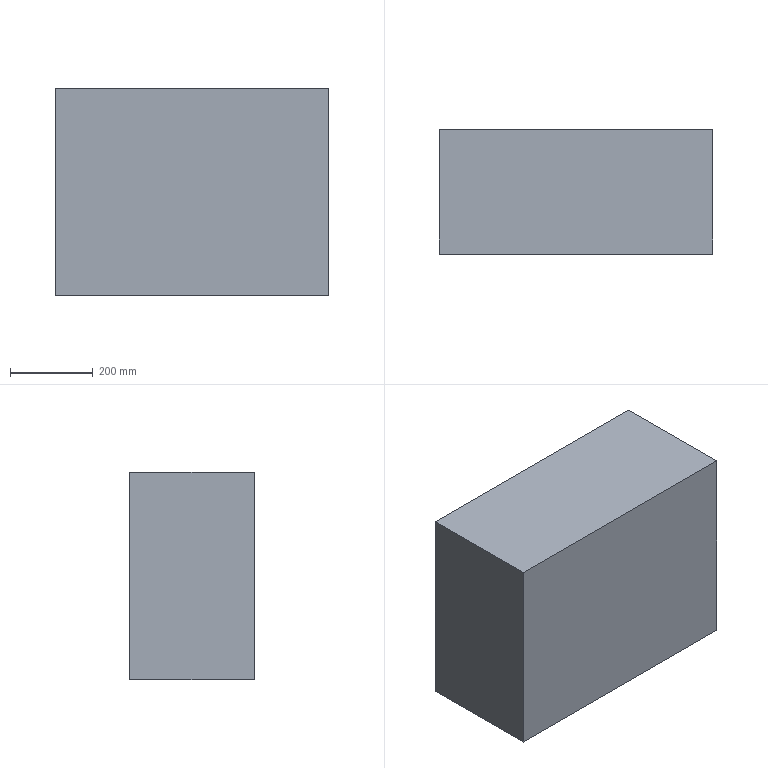Part | SolidWorks | features Extrusion 1, Shell 1 | 1 solid | 11 faces | box 660 x 300 x 500 mm | volume 11192000 mm3 | plane 11
STEP:
#1=CARTESIAN_POINT('',(-1004.904,3018.915,0.));
#2=VERTEX_POINT('',#1);
#3=CARTESIAN_POINT('',(-1004.904,2718.915,0.));
#4=VERTEX_POINT('',#3);
#5=CARTESIAN_POINT('',(-1004.904,2718.915,0.));
#6=DIRECTION('',(0.,-1.,0.));
#7=VECTOR('',#6,1000.);
#8=LINE('',#5,#7);
#9=EDGE_CURVE('',#2,#4,#8,.T.);
#10=ORIENTED_EDGE('',*,*,#9,.F.);
#11=CARTESIAN_POINT('',(-344.904,3018.915,0.));
#12=VERTEX_POINT('',#11);
#13=CARTESIAN_POINT('',(-1004.904,3018.915,0.));
#14=DIRECTION('',(-1.,0.,0.));
#15=VECTOR('',#14,1000.);
#16=LINE('',#13,#15);
#17=EDGE_CURVE('',#12,#2,#16,.T.);
#18=ORIENTED_EDGE('',*,*,#17,.F.);
#19=CARTESIAN_POINT('',(-344.904,2718.915,0.));
#20=VERTEX_POINT('',#19);
#21=CARTESIAN_POINT('',(-344.904,2718.915,0.));
#22=DIRECTION('',(0.,1.,0.));
#23=VECTOR('',#22,1000.);
#24=LINE('',#21,#23);
#25=EDGE_CURVE('',#20,#12,#24,.T.);
#26=ORIENTED_EDGE('',*,*,#25,.F.);
#27=CARTESIAN_POINT('',(-1004.904,2718.915,0.));
#28=DIRECTION('',(1.,0.,0.));
#29=VECTOR('',#28,1000.);
#30=LINE('',#27,#29);
#31=EDGE_CURVE('',#4,#20,#30,.T.);
#32=ORIENTED_EDGE('',*,*,#31,.F.);
#33=EDGE_LOOP('',(#10,#18,#26,#32));
#34=FACE_OUTER_BOUND('',#33,.T.);
#35=CARTESIAN_POINT('',(-354.904,3008.915,0.));
#36=VERTEX_POINT('',#35);
#37=CARTESIAN_POINT('',(-994.904,3008.915,0.));
#38=VERTEX_POINT('',#37);
#39=CARTESIAN_POINT('',(0.,3008.915,0.));
#40=DIRECTION('',(-1.,0.,0.));
#41=VECTOR('',#40,1000.);
#42=LINE('',#39,#41);
#43=EDGE_CURVE('',#36,#38,#42,.T.);
#44=ORIENTED_EDGE('',*,*,#43,.T.);
#45=CARTESIAN_POINT('',(-994.904,2728.915,0.));
#46=VERTEX_POINT('',#45);
#47=CARTESIAN_POINT('',(-994.904,0.,0.));
#48=DIRECTION('',(0.,-1.,0.));
#49=VECTOR('',#48,1000.);
#50=LINE('',#47,#49);
#51=EDGE_CURVE('',#38,#46,#50,.T.);
#52=ORIENTED_EDGE('',*,*,#51,.T.);
#53=CARTESIAN_POINT('',(-354.904,2728.915,0.));
#54=VERTEX_POINT('',#53);
#55=CARTESIAN_POINT('',(0.,2728.915,0.));
#56=DIRECTION('',(1.,0.,0.));
#57=VECTOR('',#56,1000.);
#58=LINE('',#55,#57);
#59=EDGE_CURVE('',#46,#54,#58,.T.);
#60=ORIENTED_EDGE('',*,*,#59,.T.);
#61=CARTESIAN_POINT('',(-354.904,0.,0.));
#62=DIRECTION('',(0.,1.,0.));
#63=VECTOR('',#62,1000.);
#64=LINE('',#61,#63);
#65=EDGE_CURVE('',#54,#36,#64,.T.);
#66=ORIENTED_EDGE('',*,*,#65,.T.);
#67=EDGE_LOOP('',(#44,#52,#60,#66));
#68=FACE_BOUND('',#67,.T.);
#69=CARTESIAN_POINT('',(0.,0.,0.));
#70=DIRECTION('',(0.,0.,-1.));
#71=DIRECTION('',(-1.,0.,0.));
#72=AXIS2_PLACEMENT_3D('',#69,#70,#71);
#73=PLANE('',#72);
#74=ADVANCED_FACE('',(#34,#68),#73,.T.);
#75=ORIENTED_EDGE('',*,*,#9,.T.);
#76=CARTESIAN_POINT('',(-1004.904,2718.915,500.));
#77=VERTEX_POINT('',#76);
#78=CARTESIAN_POINT('',(-1004.904,2718.915,500.));
#79=DIRECTION('',(0.,0.,-1.));
#80=VECTOR('',#79,1000.);
#81=LINE('',#78,#80);
#82=EDGE_CURVE('',#77,#4,#81,.T.);
#83=ORIENTED_EDGE('',*,*,#82,.F.);
#84=CARTESIAN_POINT('',(-1004.904,3018.915,500.));
#85=VERTEX_POINT('',#84);
#86=CARTESIAN_POINT('',(-1004.904,2718.915,500.));
#87=DIRECTION('',(0.,-1.,0.));
#88=VECTOR('',#87,1000.);
#89=LINE('',#86,#88);
#90=EDGE_CURVE('',#85,#77,#89,.T.);
#91=ORIENTED_EDGE('',*,*,#90,.F.);
#92=CARTESIAN_POINT('',(-1004.904,3018.915,500.));
#93=DIRECTION('',(0.,0.,-1.));
#94=VECTOR('',#93,1000.);
#95=LINE('',#92,#94);
#96=EDGE_CURVE('',#85,#2,#95,.T.);
#97=ORIENTED_EDGE('',*,*,#96,.T.);
#98=EDGE_LOOP('',(#75,#83,#91,#97));
#99=FACE_OUTER_BOUND('',#98,.T.);
#100=CARTESIAN_POINT('',(-1004.904,2718.915,500.));
#101=DIRECTION('',(1.,0.,0.));
#102=DIRECTION('',(0.,0.,-1.));
#103=AXIS2_PLACEMENT_3D('',#100,#101,#102);
#104=PLANE('',#103);
#105=ADVANCED_FACE('',(#99),#104,.F.);
#106=ORIENTED_EDGE('',*,*,#31,.T.);
#107=CARTESIAN_POINT('',(-344.904,2718.915,500.));
#108=VERTEX_POINT('',#107);
#109=CARTESIAN_POINT('',(-344.904,2718.915,500.));
#110=DIRECTION('',(0.,0.,-1.));
#111=VECTOR('',#110,1000.);
#112=LINE('',#109,#111);
#113=EDGE_CURVE('',#108,#20,#112,.T.);
#114=ORIENTED_EDGE('',*,*,#113,.F.);
#115=CARTESIAN_POINT('',(-1004.904,2718.915,500.));
#116=DIRECTION('',(1.,0.,0.));
#117=VECTOR('',#116,1000.);
#118=LINE('',#115,#117);
#119=EDGE_CURVE('',#77,#108,#118,.T.);
#120=ORIENTED_EDGE('',*,*,#119,.F.);
#121=ORIENTED_EDGE('',*,*,#82,.T.);
#122=EDGE_LOOP('',(#106,#114,#120,#121));
#123=FACE_OUTER_BOUND('',#122,.T.);
#124=CARTESIAN_POINT('',(-1004.904,2718.915,500.));
#125=DIRECTION('',(0.,1.,0.));
#126=DIRECTION('',(0.,0.,1.));
#127=AXIS2_PLACEMENT_3D('',#124,#125,#126);
#128=PLANE('',#127);
#129=ADVANCED_FACE('',(#123),#128,.F.);
#130=ORIENTED_EDGE('',*,*,#25,.T.);
#131=CARTESIAN_POINT('',(-344.904,3018.915,500.));
#132=VERTEX_POINT('',#131);
#133=CARTESIAN_POINT('',(-344.904,3018.915,500.));
#134=DIRECTION('',(0.,0.,-1.));
#135=VECTOR('',#134,1000.);
#136=LINE('',#133,#135);
#137=EDGE_CURVE('',#132,#12,#136,.T.);
#138=ORIENTED_EDGE('',*,*,#137,.F.);
#139=CARTESIAN_POINT('',(-344.904,2718.915,500.));
#140=DIRECTION('',(0.,1.,0.));
#141=VECTOR('',#140,1000.);
#142=LINE('',#139,#141);
#143=EDGE_CURVE('',#108,#132,#142,.T.);
#144=ORIENTED_EDGE('',*,*,#143,.F.);
#145=ORIENTED_EDGE('',*,*,#113,.T.);
#146=EDGE_LOOP('',(#130,#138,#144,#145));
#147=FACE_OUTER_BOUND('',#146,.T.);
#148=CARTESIAN_POINT('',(-344.904,2718.915,500.));
#149=DIRECTION('',(-1.,0.,0.));
#150=DIRECTION('',(0.,-1.,0.));
#151=AXIS2_PLACEMENT_3D('',#148,#149,#150);
#152=PLANE('',#151);
#153=ADVANCED_FACE('',(#147),#152,.F.);
#154=ORIENTED_EDGE('',*,*,#17,.T.);
#155=ORIENTED_EDGE('',*,*,#96,.F.);
#156=CARTESIAN_POINT('',(-1004.904,3018.915,500.));
#157=DIRECTION('',(-1.,0.,0.));
#158=VECTOR('',#157,1000.);
#159=LINE('',#156,#158);
#160=EDGE_CURVE('',#132,#85,#159,.T.);
#161=ORIENTED_EDGE('',*,*,#160,.F.);
#162=ORIENTED_EDGE('',*,*,#137,.T.);
#163=EDGE_LOOP('',(#154,#155,#161,#162));
#164=FACE_OUTER_BOUND('',#163,.T.);
#165=CARTESIAN_POINT('',(-1004.904,3018.915,500.));
#166=DIRECTION('',(0.,-1.,0.));
#167=DIRECTION('',(0.,0.,-1.));
#168=AXIS2_PLACEMENT_3D('',#165,#166,#167);
#169=PLANE('',#168);
#170=ADVANCED_FACE('',(#164),#169,.F.);
#171=ORIENTED_EDGE('',*,*,#90,.T.);
#172=ORIENTED_EDGE('',*,*,#119,.T.);
#173=ORIENTED_EDGE('',*,*,#143,.T.);
#174=ORIENTED_EDGE('',*,*,#160,.T.);
#175=EDGE_LOOP('',(#171,#172,#173,#174));
#176=FACE_OUTER_BOUND('',#175,.T.);
#177=CARTESIAN_POINT('',(0.,0.,500.));
#178=DIRECTION('',(0.,0.,-1.));
#179=DIRECTION('',(-1.,0.,0.));
#180=AXIS2_PLACEMENT_3D('',#177,#178,#179);
#181=PLANE('',#180);
#182=ADVANCED_FACE('',(#176),#181,.F.);
#183=ORIENTED_EDGE('',*,*,#51,.F.);
#184=CARTESIAN_POINT('',(-994.904,3008.915,490.));
#185=VERTEX_POINT('',#184);
#186=CARTESIAN_POINT('',(-994.904,3008.915,500.));
#187=DIRECTION('',(0.,0.,-1.));
#188=VECTOR('',#187,1000.);
#189=LINE('',#186,#188);
#190=EDGE_CURVE('',#185,#38,#189,.T.);
#191=ORIENTED_EDGE('',*,*,#190,.F.);
#192=CARTESIAN_POINT('',(-994.904,2728.915,490.));
#193=VERTEX_POINT('',#192);
#194=CARTESIAN_POINT('',(-994.904,0.,490.));
#195=DIRECTION('',(0.,-1.,0.));
#196=VECTOR('',#195,1000.);
#197=LINE('',#194,#196);
#198=EDGE_CURVE('',#185,#193,#197,.T.);
#199=ORIENTED_EDGE('',*,*,#198,.T.);
#200=CARTESIAN_POINT('',(-994.904,2728.915,500.));
#201=DIRECTION('',(0.,0.,-1.));
#202=VECTOR('',#201,1000.);
#203=LINE('',#200,#202);
#204=EDGE_CURVE('',#193,#46,#203,.T.);
#205=ORIENTED_EDGE('',*,*,#204,.T.);
#206=EDGE_LOOP('',(#183,#191,#199,#205));
#207=FACE_OUTER_BOUND('',#206,.T.);
#208=CARTESIAN_POINT('',(-994.904,2718.915,500.));
#209=DIRECTION('',(1.,0.,0.));
#210=DIRECTION('',(0.,0.,-1.));
#211=AXIS2_PLACEMENT_3D('',#208,#209,#210);
#212=PLANE('',#211);
#213=ADVANCED_FACE('',(#207),#212,.T.);
#214=ORIENTED_EDGE('',*,*,#59,.F.);
#215=ORIENTED_EDGE('',*,*,#204,.F.);
#216=CARTESIAN_POINT('',(-354.904,2728.915,490.));
#217=VERTEX_POINT('',#216);
#218=CARTESIAN_POINT('',(0.,2728.915,490.));
#219=DIRECTION('',(1.,0.,0.));
#220=VECTOR('',#219,1000.);
#221=LINE('',#218,#220);
#222=EDGE_CURVE('',#193,#217,#221,.T.);
#223=ORIENTED_EDGE('',*,*,#222,.T.);
#224=CARTESIAN_POINT('',(-354.904,2728.915,500.));
#225=DIRECTION('',(0.,0.,-1.));
#226=VECTOR('',#225,1000.);
#227=LINE('',#224,#226);
#228=EDGE_CURVE('',#217,#54,#227,.T.);
#229=ORIENTED_EDGE('',*,*,#228,.T.);
#230=EDGE_LOOP('',(#214,#215,#223,#229));
#231=FACE_OUTER_BOUND('',#230,.T.);
#232=CARTESIAN_POINT('',(-1004.904,2728.915,500.));
#233=DIRECTION('',(0.,1.,0.));
#234=DIRECTION('',(0.,0.,1.));
#235=AXIS2_PLACEMENT_3D('',#232,#233,#234);
#236=PLANE('',#235);
#237=ADVANCED_FACE('',(#231),#236,.T.);
#238=ORIENTED_EDGE('',*,*,#65,.F.);
#239=ORIENTED_EDGE('',*,*,#228,.F.);
#240=CARTESIAN_POINT('',(-354.904,3008.915,490.));
#241=VERTEX_POINT('',#240);
#242=CARTESIAN_POINT('',(-354.904,0.,490.));
#243=DIRECTION('',(0.,1.,0.));
#244=VECTOR('',#243,1000.);
#245=LINE('',#242,#244);
#246=EDGE_CURVE('',#217,#241,#245,.T.);
#247=ORIENTED_EDGE('',*,*,#246,.T.);
#248=CARTESIAN_POINT('',(-354.904,3008.915,500.));
#249=DIRECTION('',(0.,0.,-1.));
#250=VECTOR('',#249,1000.);
#251=LINE('',#248,#250);
#252=EDGE_CURVE('',#241,#36,#251,.T.);
#253=ORIENTED_EDGE('',*,*,#252,.T.);
#254=EDGE_LOOP('',(#238,#239,#247,#253));
#255=FACE_OUTER_BOUND('',#254,.T.);
#256=CARTESIAN_POINT('',(-354.904,2718.915,500.));
#257=DIRECTION('',(-1.,0.,0.));
#258=DIRECTION('',(0.,-1.,0.));
#259=AXIS2_PLACEMENT_3D('',#256,#257,#258);
#260=PLANE('',#259);
#261=ADVANCED_FACE('',(#255),#260,.T.);
#262=ORIENTED_EDGE('',*,*,#43,.F.);
#263=ORIENTED_EDGE('',*,*,#252,.F.);
#264=CARTESIAN_POINT('',(0.,3008.915,490.));
#265=DIRECTION('',(-1.,0.,0.));
#266=VECTOR('',#265,1000.);
#267=LINE('',#264,#266);
#268=EDGE_CURVE('',#241,#185,#267,.T.);
#269=ORIENTED_EDGE('',*,*,#268,.T.);
#270=ORIENTED_EDGE('',*,*,#190,.T.);
#271=EDGE_LOOP('',(#262,#263,#269,#270));
#272=FACE_OUTER_BOUND('',#271,.T.);
#273=CARTESIAN_POINT('',(-1004.904,3008.915,500.));
#274=DIRECTION('',(0.,-1.,0.));
#275=DIRECTION('',(0.,0.,-1.));
#276=AXIS2_PLACEMENT_3D('',#273,#274,#275);
#277=PLANE('',#276);
#278=ADVANCED_FACE('',(#272),#277,.T.);
#279=ORIENTED_EDGE('',*,*,#198,.F.);
#280=ORIENTED_EDGE('',*,*,#268,.F.);
#281=ORIENTED_EDGE('',*,*,#246,.F.);
#282=ORIENTED_EDGE('',*,*,#222,.F.);
#283=EDGE_LOOP('',(#279,#280,#281,#282));
#284=FACE_OUTER_BOUND('',#283,.T.);
#285=CARTESIAN_POINT('',(0.,0.,490.));
#286=DIRECTION('',(0.,0.,-1.));
#287=DIRECTION('',(-1.,0.,0.));
#288=AXIS2_PLACEMENT_3D('',#285,#286,#287);
#289=PLANE('',#288);
#290=ADVANCED_FACE('',(#284),#289,.T.);
#291=CLOSED_SHELL('',(#74,#105,#129,#153,#170,#182,#213,#237,#261,#278,#290));
#292=MANIFOLD_SOLID_BREP('',#291);
#293=CARTESIAN_POINT('',(0.,0.,0.));
#294=DIRECTION('',(0.,0.,1.));
#295=DIRECTION('',(1.,0.,0.));
#296=AXIS2_PLACEMENT_3D('',#293,#294,#295);
#297=(LENGTH_UNIT()NAMED_UNIT(*)SI_UNIT(.MILLI.,.METRE.));
#298=UNCERTAINTY_MEASURE_WITH_UNIT(LENGTH_MEASURE(0.00001),#297,'','');
#299=(NAMED_UNIT(*)PLANE_ANGLE_UNIT()SI_UNIT($,.RADIAN.));
#300=(NAMED_UNIT(*)SI_UNIT($,.STERADIAN.)SOLID_ANGLE_UNIT());
#301=(GEOMETRIC_REPRESENTATION_CONTEXT(3)GLOBAL_UNCERTAINTY_ASSIGNED_CONTEXT((#298))GLOBAL_UNIT_ASSIGNED_CONTEXT((#297,#299,#300))REPRESENTATION_CONTEXT('',''));
#302=ADVANCED_BREP_SHAPE_REPRESENTATION('',(#292,#296),#301);